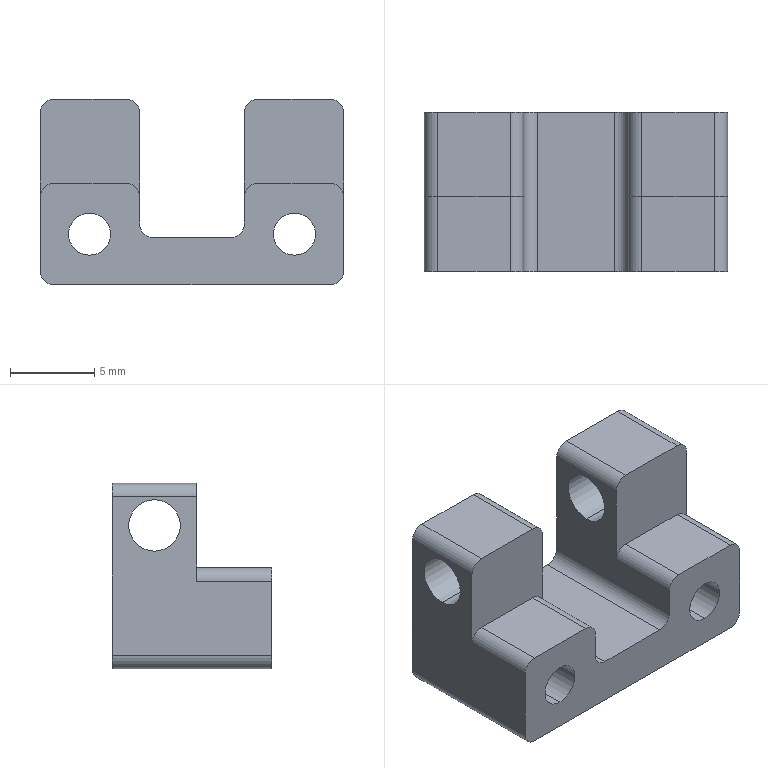Part | SolidWorks | features ICE 2, Extrusion 1, Fillet 1, HoleWzd 1 | 1 solid | 34 faces | box 18 x 9.45 x 11 mm | volume 943.932 mm3 | cylinder 20 | plane 14 | commonest cylinder face diameters 1.6 x12 2.5 x4 3.05 x4
STEP:
#1=CARTESIAN_POINT('',(-3.1,6.95,4.175));
#2=VERTEX_POINT('',#1);
#3=CARTESIAN_POINT('',(-3.1,6.95,7.225));
#4=VERTEX_POINT('',#3);
#5=CARTESIAN_POINT('',(-3.1,6.95,5.7));
#6=DIRECTION('',(-1.,0.,0.));
#7=DIRECTION('',(0.,0.,1.));
#8=AXIS2_PLACEMENT_3D('',#5,#6,#7);
#9=CIRCLE('',#8,1.525);
#10=EDGE_CURVE('',#2,#4,#9,.T.);
#11=ORIENTED_EDGE('',*,*,#10,.F.);
#12=CARTESIAN_POINT('',(-9.,6.95,4.175));
#13=VERTEX_POINT('',#12);
#14=CARTESIAN_POINT('',(9.,6.95,4.175));
#15=DIRECTION('',(-1.,0.,0.));
#16=VECTOR('',#15,1000.);
#17=LINE('',#14,#16);
#18=EDGE_CURVE('',#2,#13,#17,.T.);
#19=ORIENTED_EDGE('',*,*,#18,.T.);
#20=CARTESIAN_POINT('',(-9.,6.95,7.225));
#21=VERTEX_POINT('',#20);
#22=CARTESIAN_POINT('',(-9.,6.95,5.7));
#23=DIRECTION('',(-1.,0.,0.));
#24=DIRECTION('',(0.,0.,1.));
#25=AXIS2_PLACEMENT_3D('',#22,#23,#24);
#26=CIRCLE('',#25,1.525);
#27=EDGE_CURVE('',#13,#21,#26,.T.);
#28=ORIENTED_EDGE('',*,*,#27,.T.);
#29=CARTESIAN_POINT('',(9.,6.95,7.225));
#30=DIRECTION('',(-1.,0.,0.));
#31=VECTOR('',#30,1000.);
#32=LINE('',#29,#31);
#33=EDGE_CURVE('',#4,#21,#32,.T.);
#34=ORIENTED_EDGE('',*,*,#33,.F.);
#35=EDGE_LOOP('',(#11,#19,#28,#34));
#36=FACE_OUTER_BOUND('',#35,.T.);
#37=CARTESIAN_POINT('',(9.,6.95,5.7));
#38=DIRECTION('',(-1.,0.,0.));
#39=DIRECTION('',(0.,0.,1.));
#40=AXIS2_PLACEMENT_3D('',#37,#38,#39);
#41=CYLINDRICAL_SURFACE('',#40,1.525);
#42=ADVANCED_FACE('',(#36),#41,.F.);
#43=CARTESIAN_POINT('',(9.,6.95,4.175));
#44=VERTEX_POINT('',#43);
#45=CARTESIAN_POINT('',(9.,6.95,7.225));
#46=VERTEX_POINT('',#45);
#47=CARTESIAN_POINT('',(9.,6.95,5.7));
#48=DIRECTION('',(-1.,0.,0.));
#49=DIRECTION('',(0.,0.,1.));
#50=AXIS2_PLACEMENT_3D('',#47,#48,#49);
#51=CIRCLE('',#50,1.525);
#52=EDGE_CURVE('',#44,#46,#51,.T.);
#53=ORIENTED_EDGE('',*,*,#52,.F.);
#54=CARTESIAN_POINT('',(3.1,6.95,4.175));
#55=VERTEX_POINT('',#54);
#56=CARTESIAN_POINT('',(9.,6.95,4.175));
#57=DIRECTION('',(-1.,0.,0.));
#58=VECTOR('',#57,1000.);
#59=LINE('',#56,#58);
#60=EDGE_CURVE('',#44,#55,#59,.T.);
#61=ORIENTED_EDGE('',*,*,#60,.T.);
#62=CARTESIAN_POINT('',(3.1,6.95,7.225));
#63=VERTEX_POINT('',#62);
#64=CARTESIAN_POINT('',(3.1,6.95,5.7));
#65=DIRECTION('',(1.,0.,0.));
#66=DIRECTION('',(0.,0.,-1.));
#67=AXIS2_PLACEMENT_3D('',#64,#65,#66);
#68=CIRCLE('',#67,1.525);
#69=EDGE_CURVE('',#63,#55,#68,.T.);
#70=ORIENTED_EDGE('',*,*,#69,.F.);
#71=CARTESIAN_POINT('',(9.,6.95,7.225));
#72=DIRECTION('',(-1.,0.,0.));
#73=VECTOR('',#72,1000.);
#74=LINE('',#71,#73);
#75=EDGE_CURVE('',#46,#63,#74,.T.);
#76=ORIENTED_EDGE('',*,*,#75,.F.);
#77=EDGE_LOOP('',(#53,#61,#70,#76));
#78=FACE_OUTER_BOUND('',#77,.T.);
#79=CARTESIAN_POINT('',(9.,6.95,5.7));
#80=DIRECTION('',(-1.,0.,0.));
#81=DIRECTION('',(0.,0.,1.));
#82=AXIS2_PLACEMENT_3D('',#79,#80,#81);
#83=CYLINDRICAL_SURFACE('',#82,1.525);
#84=ADVANCED_FACE('',(#78),#83,.F.);
#85=CARTESIAN_POINT('',(-6.075,9.45,1.45));
#86=VERTEX_POINT('',#85);
#87=CARTESIAN_POINT('',(-6.075,9.45,-1.05));
#88=VERTEX_POINT('',#87);
#89=CARTESIAN_POINT('',(-6.075,9.45,0.2));
#90=DIRECTION('',(0.,-1.,0.));
#91=DIRECTION('',(0.,0.,-1.));
#92=AXIS2_PLACEMENT_3D('',#89,#90,#91);
#93=CIRCLE('',#92,1.25);
#94=EDGE_CURVE('',#86,#88,#93,.T.);
#95=ORIENTED_EDGE('',*,*,#94,.F.);
#96=CARTESIAN_POINT('',(-6.075,0.,1.45));
#97=VERTEX_POINT('',#96);
#98=CARTESIAN_POINT('',(-6.075,0.,1.45));
#99=DIRECTION('',(0.,-1.,0.));
#100=VECTOR('',#99,1000.);
#101=LINE('',#98,#100);
#102=EDGE_CURVE('',#86,#97,#101,.T.);
#103=ORIENTED_EDGE('',*,*,#102,.T.);
#104=CARTESIAN_POINT('',(-6.075,0.,-1.05));
#105=VERTEX_POINT('',#104);
#106=CARTESIAN_POINT('',(-6.075,0.,0.2));
#107=DIRECTION('',(0.,-1.,0.));
#108=DIRECTION('',(0.,0.,-1.));
#109=AXIS2_PLACEMENT_3D('',#106,#107,#108);
#110=CIRCLE('',#109,1.25);
#111=EDGE_CURVE('',#97,#105,#110,.T.);
#112=ORIENTED_EDGE('',*,*,#111,.T.);
#113=CARTESIAN_POINT('',(-6.075,0.,-1.05));
#114=DIRECTION('',(0.,-1.,0.));
#115=VECTOR('',#114,1000.);
#116=LINE('',#113,#115);
#117=EDGE_CURVE('',#88,#105,#116,.T.);
#118=ORIENTED_EDGE('',*,*,#117,.F.);
#119=EDGE_LOOP('',(#95,#103,#112,#118));
#120=FACE_OUTER_BOUND('',#119,.T.);
#121=CARTESIAN_POINT('',(-6.075,0.,0.2));
#122=DIRECTION('',(0.,-1.,0.));
#123=DIRECTION('',(0.,0.,-1.));
#124=AXIS2_PLACEMENT_3D('',#121,#122,#123);
#125=CYLINDRICAL_SURFACE('',#124,1.25);
#126=ADVANCED_FACE('',(#120),#125,.F.);
#127=CARTESIAN_POINT('',(6.075,9.45,1.45));
#128=VERTEX_POINT('',#127);
#129=CARTESIAN_POINT('',(6.075,9.45,-1.05));
#130=VERTEX_POINT('',#129);
#131=CARTESIAN_POINT('',(6.075,9.45,0.2));
#132=DIRECTION('',(0.,-1.,0.));
#133=DIRECTION('',(0.,0.,-1.));
#134=AXIS2_PLACEMENT_3D('',#131,#132,#133);
#135=CIRCLE('',#134,1.25);
#136=EDGE_CURVE('',#128,#130,#135,.T.);
#137=ORIENTED_EDGE('',*,*,#136,.F.);
#138=CARTESIAN_POINT('',(6.075,0.,1.45));
#139=VERTEX_POINT('',#138);
#140=CARTESIAN_POINT('',(6.075,0.,1.45));
#141=DIRECTION('',(0.,-1.,0.));
#142=VECTOR('',#141,1000.);
#143=LINE('',#140,#142);
#144=EDGE_CURVE('',#128,#139,#143,.T.);
#145=ORIENTED_EDGE('',*,*,#144,.T.);
#146=CARTESIAN_POINT('',(6.075,0.,-1.05));
#147=VERTEX_POINT('',#146);
#148=CARTESIAN_POINT('',(6.075,0.,0.2));
#149=DIRECTION('',(0.,-1.,0.));
#150=DIRECTION('',(0.,0.,-1.));
#151=AXIS2_PLACEMENT_3D('',#148,#149,#150);
#152=CIRCLE('',#151,1.25);
#153=EDGE_CURVE('',#139,#147,#152,.T.);
#154=ORIENTED_EDGE('',*,*,#153,.T.);
#155=CARTESIAN_POINT('',(6.075,0.,-1.05));
#156=DIRECTION('',(0.,-1.,0.));
#157=VECTOR('',#156,1000.);
#158=LINE('',#155,#157);
#159=EDGE_CURVE('',#130,#147,#158,.T.);
#160=ORIENTED_EDGE('',*,*,#159,.F.);
#161=EDGE_LOOP('',(#137,#145,#154,#160));
#162=FACE_OUTER_BOUND('',#161,.T.);
#163=CARTESIAN_POINT('',(6.075,0.,0.2));
#164=DIRECTION('',(0.,-1.,0.));
#165=DIRECTION('',(0.,0.,-1.));
#166=AXIS2_PLACEMENT_3D('',#163,#164,#165);
#167=CYLINDRICAL_SURFACE('',#166,1.25);
#168=ADVANCED_FACE('',(#162),#167,.F.);
#169=CARTESIAN_POINT('',(-9.,6.95,5.7));
#170=DIRECTION('',(-1.,0.,0.));
#171=DIRECTION('',(0.,0.,1.));
#172=AXIS2_PLACEMENT_3D('',#169,#170,#171);
#173=CIRCLE('',#172,1.525);
#174=EDGE_CURVE('',#21,#13,#173,.T.);
#175=ORIENTED_EDGE('',*,*,#174,.F.);
#176=ORIENTED_EDGE('',*,*,#27,.F.);
#177=EDGE_LOOP('',(#175,#176));
#178=FACE_BOUND('',#177,.T.);
#179=CARTESIAN_POINT('',(-9.,0.,-2.));
#180=VERTEX_POINT('',#179);
#181=CARTESIAN_POINT('',(-9.,0.,2.4));
#182=VERTEX_POINT('',#181);
#183=CARTESIAN_POINT('',(-9.,0.,3.2));
#184=DIRECTION('',(0.,0.,1.));
#185=VECTOR('',#184,1000.);
#186=LINE('',#183,#185);
#187=EDGE_CURVE('',#180,#182,#186,.T.);
#188=ORIENTED_EDGE('',*,*,#187,.T.);
#189=CARTESIAN_POINT('',(-9.,4.45,2.4));
#190=VERTEX_POINT('',#189);
#191=CARTESIAN_POINT('',(-9.,4.45,2.4));
#192=DIRECTION('',(0.,1.,0.));
#193=VECTOR('',#192,1000.);
#194=LINE('',#191,#193);
#195=EDGE_CURVE('',#182,#190,#194,.T.);
#196=ORIENTED_EDGE('',*,*,#195,.T.);
#197=CARTESIAN_POINT('',(-9.,4.45,7.4));
#198=VERTEX_POINT('',#197);
#199=CARTESIAN_POINT('',(-9.,4.45,-2.8));
#200=DIRECTION('',(0.,0.,1.));
#201=VECTOR('',#200,1000.);
#202=LINE('',#199,#201);
#203=EDGE_CURVE('',#190,#198,#202,.T.);
#204=ORIENTED_EDGE('',*,*,#203,.T.);
#205=CARTESIAN_POINT('',(-9.,9.45,7.4));
#206=VERTEX_POINT('',#205);
#207=CARTESIAN_POINT('',(-9.,4.45,7.4));
#208=DIRECTION('',(0.,1.,0.));
#209=VECTOR('',#208,1000.);
#210=LINE('',#207,#209);
#211=EDGE_CURVE('',#198,#206,#210,.T.);
#212=ORIENTED_EDGE('',*,*,#211,.T.);
#213=CARTESIAN_POINT('',(-9.,9.45,-2.));
#214=VERTEX_POINT('',#213);
#215=CARTESIAN_POINT('',(-9.,9.45,-2.8));
#216=DIRECTION('',(0.,0.,1.));
#217=VECTOR('',#216,1000.);
#218=LINE('',#215,#217);
#219=EDGE_CURVE('',#214,#206,#218,.T.);
#220=ORIENTED_EDGE('',*,*,#219,.F.);
#221=CARTESIAN_POINT('',(-9.,4.45,-2.));
#222=DIRECTION('',(0.,-1.,0.));
#223=VECTOR('',#222,1000.);
#224=LINE('',#221,#223);
#225=EDGE_CURVE('',#214,#180,#224,.T.);
#226=ORIENTED_EDGE('',*,*,#225,.T.);
#227=EDGE_LOOP('',(#188,#196,#204,#212,#220,#226));
#228=FACE_OUTER_BOUND('',#227,.T.);
#229=CARTESIAN_POINT('',(-9.,4.45,3.2));
#230=DIRECTION('',(1.,0.,0.));
#231=DIRECTION('',(0.,0.,-1.));
#232=AXIS2_PLACEMENT_3D('',#229,#230,#231);
#233=PLANE('',#232);
#234=ADVANCED_FACE('',(#178,#228),#233,.F.);
#235=CARTESIAN_POINT('',(-8.2,4.45,3.2));
#236=VERTEX_POINT('',#235);
#237=CARTESIAN_POINT('',(-3.9,4.45,3.2));
#238=VERTEX_POINT('',#237);
#239=CARTESIAN_POINT('',(-3.1,4.45,3.2));
#240=DIRECTION('',(1.,0.,0.));
#241=VECTOR('',#240,1000.);
#242=LINE('',#239,#241);
#243=EDGE_CURVE('',#236,#238,#242,.T.);
#244=ORIENTED_EDGE('',*,*,#243,.F.);
#245=CARTESIAN_POINT('',(-8.2,0.,3.2));
#246=VERTEX_POINT('',#245);
#247=CARTESIAN_POINT('',(-8.2,4.45,3.2));
#248=DIRECTION('',(0.,-1.,0.));
#249=VECTOR('',#248,1000.);
#250=LINE('',#247,#249);
#251=EDGE_CURVE('',#236,#246,#250,.T.);
#252=ORIENTED_EDGE('',*,*,#251,.T.);
#253=CARTESIAN_POINT('',(-3.9,0.,3.2));
#254=VERTEX_POINT('',#253);
#255=CARTESIAN_POINT('',(-3.1,0.,3.2));
#256=DIRECTION('',(1.,0.,0.));
#257=VECTOR('',#256,1000.);
#258=LINE('',#255,#257);
#259=EDGE_CURVE('',#246,#254,#258,.T.);
#260=ORIENTED_EDGE('',*,*,#259,.T.);
#261=CARTESIAN_POINT('',(-3.9,4.45,3.2));
#262=DIRECTION('',(0.,1.,0.));
#263=VECTOR('',#262,1000.);
#264=LINE('',#261,#263);
#265=EDGE_CURVE('',#254,#238,#264,.T.);
#266=ORIENTED_EDGE('',*,*,#265,.T.);
#267=EDGE_LOOP('',(#244,#252,#260,#266));
#268=FACE_OUTER_BOUND('',#267,.T.);
#269=CARTESIAN_POINT('',(-3.1,4.45,3.2));
#270=DIRECTION('',(0.,0.,-1.));
#271=DIRECTION('',(-1.,0.,0.));
#272=AXIS2_PLACEMENT_3D('',#269,#270,#271);
#273=PLANE('',#272);
#274=ADVANCED_FACE('',(#268),#273,.F.);
#275=CARTESIAN_POINT('',(-3.1,6.95,5.7));
#276=DIRECTION('',(-1.,0.,0.));
#277=DIRECTION('',(0.,0.,1.));
#278=AXIS2_PLACEMENT_3D('',#275,#276,#277);
#279=CIRCLE('',#278,1.525);
#280=EDGE_CURVE('',#4,#2,#279,.T.);
#281=ORIENTED_EDGE('',*,*,#280,.T.);
#282=ORIENTED_EDGE('',*,*,#10,.T.);
#283=EDGE_LOOP('',(#281,#282));
#284=FACE_BOUND('',#283,.T.);
#285=CARTESIAN_POINT('',(-3.1,4.45,7.4));
#286=VERTEX_POINT('',#285);
#287=CARTESIAN_POINT('',(-3.1,4.45,2.4));
#288=VERTEX_POINT('',#287);
#289=CARTESIAN_POINT('',(-3.1,4.45,8.2));
#290=DIRECTION('',(0.,0.,-1.));
#291=VECTOR('',#290,1000.);
#292=LINE('',#289,#291);
#293=EDGE_CURVE('',#286,#288,#292,.T.);
#294=ORIENTED_EDGE('',*,*,#293,.T.);
#295=CARTESIAN_POINT('',(-3.1,0.,2.4));
#296=VERTEX_POINT('',#295);
#297=CARTESIAN_POINT('',(-3.1,4.45,2.4));
#298=DIRECTION('',(0.,-1.,0.));
#299=VECTOR('',#298,1000.);
#300=LINE('',#297,#299);
#301=EDGE_CURVE('',#288,#296,#300,.T.);
#302=ORIENTED_EDGE('',*,*,#301,.T.);
#303=CARTESIAN_POINT('',(-3.1,0.,0.8));
#304=VERTEX_POINT('',#303);
#305=CARTESIAN_POINT('',(-3.1,0.,0.));
#306=DIRECTION('',(0.,0.,-1.));
#307=VECTOR('',#306,1000.);
#308=LINE('',#305,#307);
#309=EDGE_CURVE('',#296,#304,#308,.T.);
#310=ORIENTED_EDGE('',*,*,#309,.T.);
#311=CARTESIAN_POINT('',(-3.1,9.45,0.8));
#312=VERTEX_POINT('',#311);
#313=CARTESIAN_POINT('',(-3.1,9.45,0.8));
#314=DIRECTION('',(0.,1.,0.));
#315=VECTOR('',#314,1000.);
#316=LINE('',#313,#315);
#317=EDGE_CURVE('',#304,#312,#316,.T.);
#318=ORIENTED_EDGE('',*,*,#317,.T.);
#319=CARTESIAN_POINT('',(-3.1,9.45,7.4));
#320=VERTEX_POINT('',#319);
#321=CARTESIAN_POINT('',(-3.1,9.45,8.2));
#322=DIRECTION('',(0.,0.,-1.));
#323=VECTOR('',#322,1000.);
#324=LINE('',#321,#323);
#325=EDGE_CURVE('',#320,#312,#324,.T.);
#326=ORIENTED_EDGE('',*,*,#325,.F.);
#327=CARTESIAN_POINT('',(-3.1,4.45,7.4));
#328=DIRECTION('',(0.,-1.,0.));
#329=VECTOR('',#328,1000.);
#330=LINE('',#327,#329);
#331=EDGE_CURVE('',#320,#286,#330,.T.);
#332=ORIENTED_EDGE('',*,*,#331,.T.);
#333=EDGE_LOOP('',(#294,#302,#310,#318,#326,#332));
#334=FACE_OUTER_BOUND('',#333,.T.);
#335=CARTESIAN_POINT('',(-3.1,4.45,0.));
#336=DIRECTION('',(-1.,0.,0.));
#337=DIRECTION('',(0.,0.,1.));
#338=AXIS2_PLACEMENT_3D('',#335,#336,#337);
#339=PLANE('',#338);
#340=ADVANCED_FACE('',(#284,#334),#339,.F.);
#341=CARTESIAN_POINT('',(-2.3,0.,0.));
#342=VERTEX_POINT('',#341);
#343=CARTESIAN_POINT('',(2.3,0.,0.));
#344=VERTEX_POINT('',#343);
#345=CARTESIAN_POINT('',(3.1,0.,0.));
#346=DIRECTION('',(1.,0.,0.));
#347=VECTOR('',#346,1000.);
#348=LINE('',#345,#347);
#349=EDGE_CURVE('',#342,#344,#348,.T.);
#350=ORIENTED_EDGE('',*,*,#349,.T.);
#351=CARTESIAN_POINT('',(2.3,9.45,0.));
#352=VERTEX_POINT('',#351);
#353=CARTESIAN_POINT('',(2.3,9.45,0.));
#354=DIRECTION('',(0.,1.,0.));
#355=VECTOR('',#354,1000.);
#356=LINE('',#353,#355);
#357=EDGE_CURVE('',#344,#352,#356,.T.);
#358=ORIENTED_EDGE('',*,*,#357,.T.);
#359=CARTESIAN_POINT('',(-2.3,9.45,0.));
#360=VERTEX_POINT('',#359);
#361=CARTESIAN_POINT('',(-3.1,9.45,0.));
#362=DIRECTION('',(1.,0.,0.));
#363=VECTOR('',#362,1000.);
#364=LINE('',#361,#363);
#365=EDGE_CURVE('',#360,#352,#364,.T.);
#366=ORIENTED_EDGE('',*,*,#365,.F.);
#367=CARTESIAN_POINT('',(-2.3,0.,0.));
#368=DIRECTION('',(0.,-1.,0.));
#369=VECTOR('',#368,1000.);
#370=LINE('',#367,#369);
#371=EDGE_CURVE('',#360,#342,#370,.T.);
#372=ORIENTED_EDGE('',*,*,#371,.T.);
#373=EDGE_LOOP('',(#350,#358,#366,#372));
#374=FACE_OUTER_BOUND('',#373,.T.);
#375=CARTESIAN_POINT('',(3.1,4.45,0.));
#376=DIRECTION('',(0.,0.,-1.));
#377=DIRECTION('',(-1.,0.,0.));
#378=AXIS2_PLACEMENT_3D('',#375,#376,#377);
#379=PLANE('',#378);
#380=ADVANCED_FACE('',(#374),#379,.F.);
#381=ORIENTED_EDGE('',*,*,#69,.T.);
#382=CARTESIAN_POINT('',(3.1,6.95,5.7));
#383=DIRECTION('',(1.,0.,0.));
#384=DIRECTION('',(0.,0.,-1.));
#385=AXIS2_PLACEMENT_3D('',#382,#383,#384);
#386=CIRCLE('',#385,1.525);
#387=EDGE_CURVE('',#55,#63,#386,.T.);
#388=ORIENTED_EDGE('',*,*,#387,.T.);
#389=EDGE_LOOP('',(#381,#388));
#390=FACE_BOUND('',#389,.T.);
#391=CARTESIAN_POINT('',(3.1,0.,0.8));
#392=VERTEX_POINT('',#391);
#393=CARTESIAN_POINT('',(3.1,0.,2.4));
#394=VERTEX_POINT('',#393);
#395=CARTESIAN_POINT('',(3.1,0.,3.2));
#396=DIRECTION('',(0.,0.,1.));
#397=VECTOR('',#396,1000.);
#398=LINE('',#395,#397);
#399=EDGE_CURVE('',#392,#394,#398,.T.);
#400=ORIENTED_EDGE('',*,*,#399,.T.);
#401=CARTESIAN_POINT('',(3.1,4.45,2.4));
#402=VERTEX_POINT('',#401);
#403=CARTESIAN_POINT('',(3.1,4.45,2.4));
#404=DIRECTION('',(0.,1.,0.));
#405=VECTOR('',#404,1000.);
#406=LINE('',#403,#405);
#407=EDGE_CURVE('',#394,#402,#406,.T.);
#408=ORIENTED_EDGE('',*,*,#407,.T.);
#409=CARTESIAN_POINT('',(3.1,4.45,7.4));
#410=VERTEX_POINT('',#409);
#411=CARTESIAN_POINT('',(3.1,4.45,0.));
#412=DIRECTION('',(0.,0.,1.));
#413=VECTOR('',#412,1000.);
#414=LINE('',#411,#413);
#415=EDGE_CURVE('',#402,#410,#414,.T.);
#416=ORIENTED_EDGE('',*,*,#415,.T.);
#417=CARTESIAN_POINT('',(3.1,9.45,7.4));
#418=VERTEX_POINT('',#417);
#419=CARTESIAN_POINT('',(3.1,4.45,7.4));
#420=DIRECTION('',(0.,1.,0.));
#421=VECTOR('',#420,1000.);
#422=LINE('',#419,#421);
#423=EDGE_CURVE('',#410,#418,#422,.T.);
#424=ORIENTED_EDGE('',*,*,#423,.T.);
#425=CARTESIAN_POINT('',(3.1,9.45,0.8));
#426=VERTEX_POINT('',#425);
#427=CARTESIAN_POINT('',(3.1,9.45,0.));
#428=DIRECTION('',(0.,0.,1.));
#429=VECTOR('',#428,1000.);
#430=LINE('',#427,#429);
#431=EDGE_CURVE('',#426,#418,#430,.T.);
#432=ORIENTED_EDGE('',*,*,#431,.F.);
#433=CARTESIAN_POINT('',(3.1,0.,0.8));
#434=DIRECTION('',(0.,-1.,0.));
#435=VECTOR('',#434,1000.);
#436=LINE('',#433,#435);
#437=EDGE_CURVE('',#426,#392,#436,.T.);
#438=ORIENTED_EDGE('',*,*,#437,.T.);
#439=EDGE_LOOP('',(#400,#408,#416,#424,#432,#438));
#440=FACE_OUTER_BOUND('',#439,.T.);
#441=CARTESIAN_POINT('',(3.1,4.45,3.2));
#442=DIRECTION('',(1.,0.,0.));
#443=DIRECTION('',(0.,0.,-1.));
#444=AXIS2_PLACEMENT_3D('',#441,#442,#443);
#445=PLANE('',#444);
#446=ADVANCED_FACE('',(#390,#440),#445,.F.);
#447=CARTESIAN_POINT('',(3.9,4.45,3.2));
#448=VERTEX_POINT('',#447);
#449=CARTESIAN_POINT('',(8.2,4.45,3.2));
#450=VERTEX_POINT('',#449);
#451=CARTESIAN_POINT('',(9.,4.45,3.2));
#452=DIRECTION('',(1.,0.,0.));
#453=VECTOR('',#452,1000.);
#454=LINE('',#451,#453);
#455=EDGE_CURVE('',#448,#450,#454,.T.);
#456=ORIENTED_EDGE('',*,*,#455,.F.);
#457=CARTESIAN_POINT('',(3.9,0.,3.2));
#458=VERTEX_POINT('',#457);
#459=CARTESIAN_POINT('',(3.9,4.45,3.2));
#460=DIRECTION('',(0.,-1.,0.));
#461=VECTOR('',#460,1000.);
#462=LINE('',#459,#461);
#463=EDGE_CURVE('',#448,#458,#462,.T.);
#464=ORIENTED_EDGE('',*,*,#463,.T.);
#465=CARTESIAN_POINT('',(8.2,0.,3.2));
#466=VERTEX_POINT('',#465);
#467=CARTESIAN_POINT('',(9.,0.,3.2));
#468=DIRECTION('',(1.,0.,0.));
#469=VECTOR('',#468,1000.);
#470=LINE('',#467,#469);
#471=EDGE_CURVE('',#458,#466,#470,.T.);
#472=ORIENTED_EDGE('',*,*,#471,.T.);
#473=CARTESIAN_POINT('',(8.2,4.45,3.2));
#474=DIRECTION('',(0.,1.,0.));
#475=VECTOR('',#474,1000.);
#476=LINE('',#473,#475);
#477=EDGE_CURVE('',#466,#450,#476,.T.);
#478=ORIENTED_EDGE('',*,*,#477,.T.);
#479=EDGE_LOOP('',(#456,#464,#472,#478));
#480=FACE_OUTER_BOUND('',#479,.T.);
#481=CARTESIAN_POINT('',(9.,4.45,3.2));
#482=DIRECTION('',(0.,0.,-1.));
#483=DIRECTION('',(-1.,0.,0.));
#484=AXIS2_PLACEMENT_3D('',#481,#482,#483);
#485=PLANE('',#484);
#486=ADVANCED_FACE('',(#480),#485,.F.);
#487=CARTESIAN_POINT('',(9.,6.95,5.7));
#488=DIRECTION('',(-1.,0.,0.));
#489=DIRECTION('',(0.,0.,1.));
#490=AXIS2_PLACEMENT_3D('',#487,#488,#489);
#491=CIRCLE('',#490,1.525);
#492=EDGE_CURVE('',#46,#44,#491,.T.);
#493=ORIENTED_EDGE('',*,*,#492,.T.);
#494=ORIENTED_EDGE('',*,*,#52,.T.);
#495=EDGE_LOOP('',(#493,#494));
#496=FACE_BOUND('',#495,.T.);
#497=CARTESIAN_POINT('',(9.,4.45,7.4));
#498=VERTEX_POINT('',#497);
#499=CARTESIAN_POINT('',(9.,4.45,2.4));
#500=VERTEX_POINT('',#499);
#501=CARTESIAN_POINT('',(9.,4.45,8.2));
#502=DIRECTION('',(0.,0.,-1.));
#503=VECTOR('',#502,1000.);
#504=LINE('',#501,#503);
#505=EDGE_CURVE('',#498,#500,#504,.T.);
#506=ORIENTED_EDGE('',*,*,#505,.T.);
#507=CARTESIAN_POINT('',(9.,0.,2.4));
#508=VERTEX_POINT('',#507);
#509=CARTESIAN_POINT('',(9.,4.45,2.4));
#510=DIRECTION('',(0.,-1.,0.));
#511=VECTOR('',#510,1000.);
#512=LINE('',#509,#511);
#513=EDGE_CURVE('',#500,#508,#512,.T.);
#514=ORIENTED_EDGE('',*,*,#513,.T.);
#515=CARTESIAN_POINT('',(9.,0.,-2.));
#516=VERTEX_POINT('',#515);
#517=CARTESIAN_POINT('',(9.,0.,-2.8));
#518=DIRECTION('',(0.,0.,-1.));
#519=VECTOR('',#518,1000.);
#520=LINE('',#517,#519);
#521=EDGE_CURVE('',#508,#516,#520,.T.);
#522=ORIENTED_EDGE('',*,*,#521,.T.);
#523=CARTESIAN_POINT('',(9.,9.45,-2.));
#524=VERTEX_POINT('',#523);
#525=CARTESIAN_POINT('',(9.,4.45,-2.));
#526=DIRECTION('',(0.,1.,0.));
#527=VECTOR('',#526,1000.);
#528=LINE('',#525,#527);
#529=EDGE_CURVE('',#516,#524,#528,.T.);
#530=ORIENTED_EDGE('',*,*,#529,.T.);
#531=CARTESIAN_POINT('',(9.,9.45,7.4));
#532=VERTEX_POINT('',#531);
#533=CARTESIAN_POINT('',(9.,9.45,8.2));
#534=DIRECTION('',(0.,0.,-1.));
#535=VECTOR('',#534,1000.);
#536=LINE('',#533,#535);
#537=EDGE_CURVE('',#532,#524,#536,.T.);
#538=ORIENTED_EDGE('',*,*,#537,.F.);
#539=CARTESIAN_POINT('',(9.,4.45,7.4));
#540=DIRECTION('',(0.,-1.,0.));
#541=VECTOR('',#540,1000.);
#542=LINE('',#539,#541);
#543=EDGE_CURVE('',#532,#498,#542,.T.);
#544=ORIENTED_EDGE('',*,*,#543,.T.);
#545=EDGE_LOOP('',(#506,#514,#522,#530,#538,#544));
#546=FACE_OUTER_BOUND('',#545,.T.);
#547=CARTESIAN_POINT('',(9.,4.45,-2.8));
#548=DIRECTION('',(-1.,0.,0.));
#549=DIRECTION('',(0.,0.,1.));
#550=AXIS2_PLACEMENT_3D('',#547,#548,#549);
#551=PLANE('',#550);
#552=ADVANCED_FACE('',(#496,#546),#551,.F.);
#553=CARTESIAN_POINT('',(8.2,0.,-2.8));
#554=VERTEX_POINT('',#553);
#555=CARTESIAN_POINT('',(-8.2,0.,-2.8));
#556=VERTEX_POINT('',#555);
#557=CARTESIAN_POINT('',(-9.,0.,-2.8));
#558=DIRECTION('',(-1.,0.,0.));
#559=VECTOR('',#558,1000.);
#560=LINE('',#557,#559);
#561=EDGE_CURVE('',#554,#556,#560,.T.);
#562=ORIENTED_EDGE('',*,*,#561,.T.);
#563=CARTESIAN_POINT('',(-8.2,9.45,-2.8));
#564=VERTEX_POINT('',#563);
#565=CARTESIAN_POINT('',(-8.2,4.45,-2.8));
#566=DIRECTION('',(0.,1.,0.));
#567=VECTOR('',#566,1000.);
#568=LINE('',#565,#567);
#569=EDGE_CURVE('',#556,#564,#568,.T.);
#570=ORIENTED_EDGE('',*,*,#569,.T.);
#571=CARTESIAN_POINT('',(8.2,9.45,-2.8));
#572=VERTEX_POINT('',#571);
#573=CARTESIAN_POINT('',(9.,9.45,-2.8));
#574=DIRECTION('',(-1.,0.,0.));
#575=VECTOR('',#574,1000.);
#576=LINE('',#573,#575);
#577=EDGE_CURVE('',#572,#564,#576,.T.);
#578=ORIENTED_EDGE('',*,*,#577,.F.);
#579=CARTESIAN_POINT('',(8.2,4.45,-2.8));
#580=DIRECTION('',(0.,-1.,0.));
#581=VECTOR('',#580,1000.);
#582=LINE('',#579,#581);
#583=EDGE_CURVE('',#572,#554,#582,.T.);
#584=ORIENTED_EDGE('',*,*,#583,.T.);
#585=EDGE_LOOP('',(#562,#570,#578,#584));
#586=FACE_OUTER_BOUND('',#585,.T.);
#587=CARTESIAN_POINT('',(-9.,4.45,-2.8));
#588=DIRECTION('',(0.,0.,1.));
#589=DIRECTION('',(1.,0.,0.));
#590=AXIS2_PLACEMENT_3D('',#587,#588,#589);
#591=PLANE('',#590);
#592=ADVANCED_FACE('',(#586),#591,.F.);
#593=CARTESIAN_POINT('',(-6.075,0.,0.2));
#594=DIRECTION('',(0.,-1.,0.));
#595=DIRECTION('',(0.,0.,-1.));
#596=AXIS2_PLACEMENT_3D('',#593,#594,#595);
#597=CIRCLE('',#596,1.25);
#598=EDGE_CURVE('',#105,#97,#597,.T.);
#599=ORIENTED_EDGE('',*,*,#598,.F.);
#600=ORIENTED_EDGE('',*,*,#111,.F.);
#601=EDGE_LOOP('',(#599,#600));
#602=FACE_BOUND('',#601,.T.);
#603=CARTESIAN_POINT('',(6.075,0.,0.2));
#604=DIRECTION('',(0.,-1.,0.));
#605=DIRECTION('',(0.,0.,-1.));
#606=AXIS2_PLACEMENT_3D('',#603,#604,#605);
#607=CIRCLE('',#606,1.25);
#608=EDGE_CURVE('',#147,#139,#607,.T.);
#609=ORIENTED_EDGE('',*,*,#608,.F.);
#610=ORIENTED_EDGE('',*,*,#153,.F.);
#611=EDGE_LOOP('',(#609,#610));
#612=FACE_BOUND('',#611,.T.);
#613=ORIENTED_EDGE('',*,*,#259,.F.);
#614=CARTESIAN_POINT('',(-8.2,0.,2.4));
#615=DIRECTION('',(0.,-1.,0.));
#616=DIRECTION('',(0.,0.,-1.));
#617=AXIS2_PLACEMENT_3D('',#614,#615,#616);
#618=CIRCLE('',#617,0.8);
#619=EDGE_CURVE('',#246,#182,#618,.T.);
#620=ORIENTED_EDGE('',*,*,#619,.T.);
#621=ORIENTED_EDGE('',*,*,#187,.F.);
#622=CARTESIAN_POINT('',(-8.2,0.,-2.));
#623=DIRECTION('',(0.,-1.,0.));
#624=DIRECTION('',(0.,0.,-1.));
#625=AXIS2_PLACEMENT_3D('',#622,#623,#624);
#626=CIRCLE('',#625,0.8);
#627=EDGE_CURVE('',#180,#556,#626,.T.);
#628=ORIENTED_EDGE('',*,*,#627,.T.);
#629=ORIENTED_EDGE('',*,*,#561,.F.);
#630=CARTESIAN_POINT('',(8.2,0.,-2.));
#631=DIRECTION('',(0.,-1.,0.));
#632=DIRECTION('',(0.,0.,-1.));
#633=AXIS2_PLACEMENT_3D('',#630,#631,#632);
#634=CIRCLE('',#633,0.8);
#635=EDGE_CURVE('',#554,#516,#634,.T.);
#636=ORIENTED_EDGE('',*,*,#635,.T.);
#637=ORIENTED_EDGE('',*,*,#521,.F.);
#638=CARTESIAN_POINT('',(8.2,0.,2.4));
#639=DIRECTION('',(0.,-1.,0.));
#640=DIRECTION('',(0.,0.,-1.));
#641=AXIS2_PLACEMENT_3D('',#638,#639,#640);
#642=CIRCLE('',#641,0.8);
#643=EDGE_CURVE('',#508,#466,#642,.T.);
#644=ORIENTED_EDGE('',*,*,#643,.T.);
#645=ORIENTED_EDGE('',*,*,#471,.F.);
#646=CARTESIAN_POINT('',(3.9,0.,2.4));
#647=DIRECTION('',(0.,-1.,0.));
#648=DIRECTION('',(0.,0.,-1.));
#649=AXIS2_PLACEMENT_3D('',#646,#647,#648);
#650=CIRCLE('',#649,0.8);
#651=EDGE_CURVE('',#458,#394,#650,.T.);
#652=ORIENTED_EDGE('',*,*,#651,.T.);
#653=ORIENTED_EDGE('',*,*,#399,.F.);
#654=CARTESIAN_POINT('',(2.3,0.,0.8));
#655=DIRECTION('',(0.,1.,0.));
#656=DIRECTION('',(0.,0.,-1.));
#657=AXIS2_PLACEMENT_3D('',#654,#655,#656);
#658=CIRCLE('',#657,0.8);
#659=EDGE_CURVE('',#392,#344,#658,.T.);
#660=ORIENTED_EDGE('',*,*,#659,.T.);
#661=ORIENTED_EDGE('',*,*,#349,.F.);
#662=CARTESIAN_POINT('',(-2.3,0.,0.8));
#663=DIRECTION('',(0.,1.,0.));
#664=DIRECTION('',(0.,0.,-1.));
#665=AXIS2_PLACEMENT_3D('',#662,#663,#664);
#666=CIRCLE('',#665,0.8);
#667=EDGE_CURVE('',#342,#304,#666,.T.);
#668=ORIENTED_EDGE('',*,*,#667,.T.);
#669=ORIENTED_EDGE('',*,*,#309,.F.);
#670=CARTESIAN_POINT('',(-3.9,0.,2.4));
#671=DIRECTION('',(0.,-1.,0.));
#672=DIRECTION('',(0.,0.,-1.));
#673=AXIS2_PLACEMENT_3D('',#670,#671,#672);
#674=CIRCLE('',#673,0.8);
#675=EDGE_CURVE('',#296,#254,#674,.T.);
#676=ORIENTED_EDGE('',*,*,#675,.T.);
#677=EDGE_LOOP('',(#613,#620,#621,#628,#629,#636,#637,#644,#645,#652,#653,#660,#661,#668,#669,#676));
#678=FACE_OUTER_BOUND('',#677,.T.);
#679=CARTESIAN_POINT('',(0.,0.,0.));
#680=DIRECTION('',(0.,-1.,0.));
#681=DIRECTION('',(0.,0.,-1.));
#682=AXIS2_PLACEMENT_3D('',#679,#680,#681);
#683=PLANE('',#682);
#684=ADVANCED_FACE('',(#602,#612,#678),#683,.T.);
#685=ORIENTED_EDGE('',*,*,#293,.F.);
#686=CARTESIAN_POINT('',(-3.9,4.45,8.2));
#687=VERTEX_POINT('',#686);
#688=CARTESIAN_POINT('',(-3.9,4.45,7.4));
#689=DIRECTION('',(0.,-1.,0.));
#690=DIRECTION('',(0.,0.,1.));
#691=AXIS2_PLACEMENT_3D('',#688,#689,#690);
#692=CIRCLE('',#691,0.8);
#693=EDGE_CURVE('',#286,#687,#692,.T.);
#694=ORIENTED_EDGE('',*,*,#693,.T.);
#695=CARTESIAN_POINT('',(-8.2,4.45,8.2));
#696=VERTEX_POINT('',#695);
#697=CARTESIAN_POINT('',(-9.,4.45,8.2));
#698=DIRECTION('',(1.,0.,0.));
#699=VECTOR('',#698,1000.);
#700=LINE('',#697,#699);
#701=EDGE_CURVE('',#696,#687,#700,.T.);
#702=ORIENTED_EDGE('',*,*,#701,.F.);
#703=CARTESIAN_POINT('',(-8.2,4.45,7.4));
#704=DIRECTION('',(0.,-1.,0.));
#705=DIRECTION('',(0.,0.,1.));
#706=AXIS2_PLACEMENT_3D('',#703,#704,#705);
#707=CIRCLE('',#706,0.8);
#708=EDGE_CURVE('',#696,#198,#707,.T.);
#709=ORIENTED_EDGE('',*,*,#708,.T.);
#710=ORIENTED_EDGE('',*,*,#203,.F.);
#711=CARTESIAN_POINT('',(-8.2,4.45,2.4));
#712=DIRECTION('',(0.,1.,0.));
#713=DIRECTION('',(0.,0.,1.));
#714=AXIS2_PLACEMENT_3D('',#711,#712,#713);
#715=CIRCLE('',#714,0.8);
#716=EDGE_CURVE('',#190,#236,#715,.T.);
#717=ORIENTED_EDGE('',*,*,#716,.T.);
#718=ORIENTED_EDGE('',*,*,#243,.T.);
#719=CARTESIAN_POINT('',(-3.9,4.45,2.4));
#720=DIRECTION('',(0.,1.,0.));
#721=DIRECTION('',(0.,0.,1.));
#722=AXIS2_PLACEMENT_3D('',#719,#720,#721);
#723=CIRCLE('',#722,0.8);
#724=EDGE_CURVE('',#238,#288,#723,.T.);
#725=ORIENTED_EDGE('',*,*,#724,.T.);
#726=EDGE_LOOP('',(#685,#694,#702,#709,#710,#717,#718,#725));
#727=FACE_OUTER_BOUND('',#726,.T.);
#728=CARTESIAN_POINT('',(0.,4.45,0.));
#729=DIRECTION('',(0.,1.,0.));
#730=DIRECTION('',(0.,0.,1.));
#731=AXIS2_PLACEMENT_3D('',#728,#729,#730);
#732=PLANE('',#731);
#733=ADVANCED_FACE('',(#727),#732,.F.);
#734=ORIENTED_EDGE('',*,*,#505,.F.);
#735=CARTESIAN_POINT('',(8.2,4.45,8.2));
#736=VERTEX_POINT('',#735);
#737=CARTESIAN_POINT('',(8.2,4.45,7.4));
#738=DIRECTION('',(0.,-1.,0.));
#739=DIRECTION('',(0.,0.,1.));
#740=AXIS2_PLACEMENT_3D('',#737,#738,#739);
#741=CIRCLE('',#740,0.8);
#742=EDGE_CURVE('',#498,#736,#741,.T.);
#743=ORIENTED_EDGE('',*,*,#742,.T.);
#744=CARTESIAN_POINT('',(3.9,4.45,8.2));
#745=VERTEX_POINT('',#744);
#746=CARTESIAN_POINT('',(3.1,4.45,8.2));
#747=DIRECTION('',(1.,0.,0.));
#748=VECTOR('',#747,1000.);
#749=LINE('',#746,#748);
#750=EDGE_CURVE('',#745,#736,#749,.T.);
#751=ORIENTED_EDGE('',*,*,#750,.F.);
#752=CARTESIAN_POINT('',(3.9,4.45,7.4));
#753=DIRECTION('',(0.,-1.,0.));
#754=DIRECTION('',(0.,0.,1.));
#755=AXIS2_PLACEMENT_3D('',#752,#753,#754);
#756=CIRCLE('',#755,0.8);
#757=EDGE_CURVE('',#745,#410,#756,.T.);
#758=ORIENTED_EDGE('',*,*,#757,.T.);
#759=ORIENTED_EDGE('',*,*,#415,.F.);
#760=CARTESIAN_POINT('',(3.9,4.45,2.4));
#761=DIRECTION('',(0.,1.,0.));
#762=DIRECTION('',(0.,0.,1.));
#763=AXIS2_PLACEMENT_3D('',#760,#761,#762);
#764=CIRCLE('',#763,0.8);
#765=EDGE_CURVE('',#402,#448,#764,.T.);
#766=ORIENTED_EDGE('',*,*,#765,.T.);
#767=ORIENTED_EDGE('',*,*,#455,.T.);
#768=CARTESIAN_POINT('',(8.2,4.45,2.4));
#769=DIRECTION('',(0.,1.,0.));
#770=DIRECTION('',(0.,0.,1.));
#771=AXIS2_PLACEMENT_3D('',#768,#769,#770);
#772=CIRCLE('',#771,0.8);
#773=EDGE_CURVE('',#450,#500,#772,.T.);
#774=ORIENTED_EDGE('',*,*,#773,.T.);
#775=EDGE_LOOP('',(#734,#743,#751,#758,#759,#766,#767,#774));
#776=FACE_OUTER_BOUND('',#775,.T.);
#777=CARTESIAN_POINT('',(0.,4.45,0.));
#778=DIRECTION('',(0.,1.,0.));
#779=DIRECTION('',(0.,0.,1.));
#780=AXIS2_PLACEMENT_3D('',#777,#778,#779);
#781=PLANE('',#780);
#782=ADVANCED_FACE('',(#776),#781,.F.);
#783=ORIENTED_EDGE('',*,*,#701,.T.);
#784=CARTESIAN_POINT('',(-3.9,9.45,8.2));
#785=VERTEX_POINT('',#784);
#786=CARTESIAN_POINT('',(-3.9,9.45,8.2));
#787=DIRECTION('',(0.,1.,0.));
#788=VECTOR('',#787,1000.);
#789=LINE('',#786,#788);
#790=EDGE_CURVE('',#687,#785,#789,.T.);
#791=ORIENTED_EDGE('',*,*,#790,.T.);
#792=CARTESIAN_POINT('',(-8.2,9.45,8.2));
#793=VERTEX_POINT('',#792);
#794=CARTESIAN_POINT('',(-9.,9.45,8.2));
#795=DIRECTION('',(1.,0.,0.));
#796=VECTOR('',#795,1000.);
#797=LINE('',#794,#796);
#798=EDGE_CURVE('',#793,#785,#797,.T.);
#799=ORIENTED_EDGE('',*,*,#798,.F.);
#800=CARTESIAN_POINT('',(-8.2,9.45,8.2));
#801=DIRECTION('',(0.,-1.,0.));
#802=VECTOR('',#801,1000.);
#803=LINE('',#800,#802);
#804=EDGE_CURVE('',#793,#696,#803,.T.);
#805=ORIENTED_EDGE('',*,*,#804,.T.);
#806=EDGE_LOOP('',(#783,#791,#799,#805));
#807=FACE_OUTER_BOUND('',#806,.T.);
#808=CARTESIAN_POINT('',(-9.,9.45,8.2));
#809=DIRECTION('',(0.,0.,-1.));
#810=DIRECTION('',(-1.,0.,0.));
#811=AXIS2_PLACEMENT_3D('',#808,#809,#810);
#812=PLANE('',#811);
#813=ADVANCED_FACE('',(#807),#812,.F.);
#814=ORIENTED_EDGE('',*,*,#750,.T.);
#815=CARTESIAN_POINT('',(8.2,9.45,8.2));
#816=VERTEX_POINT('',#815);
#817=CARTESIAN_POINT('',(8.2,9.45,8.2));
#818=DIRECTION('',(0.,1.,0.));
#819=VECTOR('',#818,1000.);
#820=LINE('',#817,#819);
#821=EDGE_CURVE('',#736,#816,#820,.T.);
#822=ORIENTED_EDGE('',*,*,#821,.T.);
#823=CARTESIAN_POINT('',(3.9,9.45,8.2));
#824=VERTEX_POINT('',#823);
#825=CARTESIAN_POINT('',(3.1,9.45,8.2));
#826=DIRECTION('',(1.,0.,0.));
#827=VECTOR('',#826,1000.);
#828=LINE('',#825,#827);
#829=EDGE_CURVE('',#824,#816,#828,.T.);
#830=ORIENTED_EDGE('',*,*,#829,.F.);
#831=CARTESIAN_POINT('',(3.9,9.45,8.2));
#832=DIRECTION('',(0.,-1.,0.));
#833=VECTOR('',#832,1000.);
#834=LINE('',#831,#833);
#835=EDGE_CURVE('',#824,#745,#834,.T.);
#836=ORIENTED_EDGE('',*,*,#835,.T.);
#837=EDGE_LOOP('',(#814,#822,#830,#836));
#838=FACE_OUTER_BOUND('',#837,.T.);
#839=CARTESIAN_POINT('',(3.1,9.45,8.2));
#840=DIRECTION('',(0.,0.,-1.));
#841=DIRECTION('',(-1.,0.,0.));
#842=AXIS2_PLACEMENT_3D('',#839,#840,#841);
#843=PLANE('',#842);
#844=ADVANCED_FACE('',(#838),#843,.F.);
#845=CARTESIAN_POINT('',(-6.075,9.45,0.2));
#846=DIRECTION('',(0.,-1.,0.));
#847=DIRECTION('',(0.,0.,-1.));
#848=AXIS2_PLACEMENT_3D('',#845,#846,#847);
#849=CIRCLE('',#848,1.25);
#850=EDGE_CURVE('',#88,#86,#849,.T.);
#851=ORIENTED_EDGE('',*,*,#850,.T.);
#852=ORIENTED_EDGE('',*,*,#94,.T.);
#853=EDGE_LOOP('',(#851,#852));
#854=FACE_BOUND('',#853,.T.);
#855=CARTESIAN_POINT('',(6.075,9.45,0.2));
#856=DIRECTION('',(0.,-1.,0.));
#857=DIRECTION('',(0.,0.,-1.));
#858=AXIS2_PLACEMENT_3D('',#855,#856,#857);
#859=CIRCLE('',#858,1.25);
#860=EDGE_CURVE('',#130,#128,#859,.T.);
#861=ORIENTED_EDGE('',*,*,#860,.T.);
#862=ORIENTED_EDGE('',*,*,#136,.T.);
#863=EDGE_LOOP('',(#861,#862));
#864=FACE_BOUND('',#863,.T.);
#865=ORIENTED_EDGE('',*,*,#577,.T.);
#866=CARTESIAN_POINT('',(-8.2,9.45,-2.));
#867=DIRECTION('',(0.,1.,0.));
#868=DIRECTION('',(0.,0.,1.));
#869=AXIS2_PLACEMENT_3D('',#866,#867,#868);
#870=CIRCLE('',#869,0.8);
#871=EDGE_CURVE('',#564,#214,#870,.T.);
#872=ORIENTED_EDGE('',*,*,#871,.T.);
#873=ORIENTED_EDGE('',*,*,#219,.T.);
#874=CARTESIAN_POINT('',(-8.2,9.45,7.4));
#875=DIRECTION('',(0.,1.,0.));
#876=DIRECTION('',(0.,0.,1.));
#877=AXIS2_PLACEMENT_3D('',#874,#875,#876);
#878=CIRCLE('',#877,0.8);
#879=EDGE_CURVE('',#206,#793,#878,.T.);
#880=ORIENTED_EDGE('',*,*,#879,.T.);
#881=ORIENTED_EDGE('',*,*,#798,.T.);
#882=CARTESIAN_POINT('',(-3.9,9.45,7.4));
#883=DIRECTION('',(0.,1.,0.));
#884=DIRECTION('',(0.,0.,1.));
#885=AXIS2_PLACEMENT_3D('',#882,#883,#884);
#886=CIRCLE('',#885,0.8);
#887=EDGE_CURVE('',#785,#320,#886,.T.);
#888=ORIENTED_EDGE('',*,*,#887,.T.);
#889=ORIENTED_EDGE('',*,*,#325,.T.);
#890=CARTESIAN_POINT('',(-2.3,9.45,0.8));
#891=DIRECTION('',(0.,-1.,0.));
#892=DIRECTION('',(0.,0.,1.));
#893=AXIS2_PLACEMENT_3D('',#890,#891,#892);
#894=CIRCLE('',#893,0.8);
#895=EDGE_CURVE('',#312,#360,#894,.T.);
#896=ORIENTED_EDGE('',*,*,#895,.T.);
#897=ORIENTED_EDGE('',*,*,#365,.T.);
#898=CARTESIAN_POINT('',(2.3,9.45,0.8));
#899=DIRECTION('',(0.,-1.,0.));
#900=DIRECTION('',(0.,0.,1.));
#901=AXIS2_PLACEMENT_3D('',#898,#899,#900);
#902=CIRCLE('',#901,0.8);
#903=EDGE_CURVE('',#352,#426,#902,.T.);
#904=ORIENTED_EDGE('',*,*,#903,.T.);
#905=ORIENTED_EDGE('',*,*,#431,.T.);
#906=CARTESIAN_POINT('',(3.9,9.45,7.4));
#907=DIRECTION('',(0.,1.,0.));
#908=DIRECTION('',(0.,0.,1.));
#909=AXIS2_PLACEMENT_3D('',#906,#907,#908);
#910=CIRCLE('',#909,0.8);
#911=EDGE_CURVE('',#418,#824,#910,.T.);
#912=ORIENTED_EDGE('',*,*,#911,.T.);
#913=ORIENTED_EDGE('',*,*,#829,.T.);
#914=CARTESIAN_POINT('',(8.2,9.45,7.4));
#915=DIRECTION('',(0.,1.,0.));
#916=DIRECTION('',(0.,0.,1.));
#917=AXIS2_PLACEMENT_3D('',#914,#915,#916);
#918=CIRCLE('',#917,0.8);
#919=EDGE_CURVE('',#816,#532,#918,.T.);
#920=ORIENTED_EDGE('',*,*,#919,.T.);
#921=ORIENTED_EDGE('',*,*,#537,.T.);
#922=CARTESIAN_POINT('',(8.2,9.45,-2.));
#923=DIRECTION('',(0.,1.,0.));
#924=DIRECTION('',(0.,0.,1.));
#925=AXIS2_PLACEMENT_3D('',#922,#923,#924);
#926=CIRCLE('',#925,0.8);
#927=EDGE_CURVE('',#524,#572,#926,.T.);
#928=ORIENTED_EDGE('',*,*,#927,.T.);
#929=EDGE_LOOP('',(#865,#872,#873,#880,#881,#888,#889,#896,#897,#904,#905,#912,#913,#920,#921,#928));
#930=FACE_OUTER_BOUND('',#929,.T.);
#931=CARTESIAN_POINT('',(0.,9.45,0.));
#932=DIRECTION('',(0.,1.,0.));
#933=DIRECTION('',(0.,0.,1.));
#934=AXIS2_PLACEMENT_3D('',#931,#932,#933);
#935=PLANE('',#934);
#936=ADVANCED_FACE('',(#854,#864,#930),#935,.T.);
#937=ORIENTED_EDGE('',*,*,#144,.F.);
#938=ORIENTED_EDGE('',*,*,#860,.F.);
#939=ORIENTED_EDGE('',*,*,#159,.T.);
#940=ORIENTED_EDGE('',*,*,#608,.T.);
#941=EDGE_LOOP('',(#937,#938,#939,#940));
#942=FACE_OUTER_BOUND('',#941,.T.);
#943=CARTESIAN_POINT('',(6.075,0.,0.2));
#944=DIRECTION('',(0.,-1.,0.));
#945=DIRECTION('',(0.,0.,-1.));
#946=AXIS2_PLACEMENT_3D('',#943,#944,#945);
#947=CYLINDRICAL_SURFACE('',#946,1.25);
#948=ADVANCED_FACE('',(#942),#947,.F.);
#949=ORIENTED_EDGE('',*,*,#102,.F.);
#950=ORIENTED_EDGE('',*,*,#850,.F.);
#951=ORIENTED_EDGE('',*,*,#117,.T.);
#952=ORIENTED_EDGE('',*,*,#598,.T.);
#953=EDGE_LOOP('',(#949,#950,#951,#952));
#954=FACE_OUTER_BOUND('',#953,.T.);
#955=CARTESIAN_POINT('',(-6.075,0.,0.2));
#956=DIRECTION('',(0.,-1.,0.));
#957=DIRECTION('',(0.,0.,-1.));
#958=AXIS2_PLACEMENT_3D('',#955,#956,#957);
#959=CYLINDRICAL_SURFACE('',#958,1.25);
#960=ADVANCED_FACE('',(#954),#959,.F.);
#961=ORIENTED_EDGE('',*,*,#60,.F.);
#962=ORIENTED_EDGE('',*,*,#492,.F.);
#963=ORIENTED_EDGE('',*,*,#75,.T.);
#964=ORIENTED_EDGE('',*,*,#387,.F.);
#965=EDGE_LOOP('',(#961,#962,#963,#964));
#966=FACE_OUTER_BOUND('',#965,.T.);
#967=CARTESIAN_POINT('',(9.,6.95,5.7));
#968=DIRECTION('',(-1.,0.,0.));
#969=DIRECTION('',(0.,0.,1.));
#970=AXIS2_PLACEMENT_3D('',#967,#968,#969);
#971=CYLINDRICAL_SURFACE('',#970,1.525);
#972=ADVANCED_FACE('',(#966),#971,.F.);
#973=ORIENTED_EDGE('',*,*,#18,.F.);
#974=ORIENTED_EDGE('',*,*,#280,.F.);
#975=ORIENTED_EDGE('',*,*,#33,.T.);
#976=ORIENTED_EDGE('',*,*,#174,.T.);
#977=EDGE_LOOP('',(#973,#974,#975,#976));
#978=FACE_OUTER_BOUND('',#977,.T.);
#979=CARTESIAN_POINT('',(9.,6.95,5.7));
#980=DIRECTION('',(-1.,0.,0.));
#981=DIRECTION('',(0.,0.,1.));
#982=AXIS2_PLACEMENT_3D('',#979,#980,#981);
#983=CYLINDRICAL_SURFACE('',#982,1.525);
#984=ADVANCED_FACE('',(#978),#983,.F.);
#985=ORIENTED_EDGE('',*,*,#716,.F.);
#986=ORIENTED_EDGE('',*,*,#195,.F.);
#987=ORIENTED_EDGE('',*,*,#619,.F.);
#988=ORIENTED_EDGE('',*,*,#251,.F.);
#989=EDGE_LOOP('',(#985,#986,#987,#988));
#990=FACE_OUTER_BOUND('',#989,.T.);
#991=CARTESIAN_POINT('',(-8.2,4.45,2.4));
#992=DIRECTION('',(0.,-1.,0.));
#993=DIRECTION('',(0.,0.,-1.));
#994=AXIS2_PLACEMENT_3D('',#991,#992,#993);
#995=CYLINDRICAL_SURFACE('',#994,0.8);
#996=ADVANCED_FACE('',(#990),#995,.T.);
#997=ORIENTED_EDGE('',*,*,#724,.F.);
#998=ORIENTED_EDGE('',*,*,#265,.F.);
#999=ORIENTED_EDGE('',*,*,#675,.F.);
#1000=ORIENTED_EDGE('',*,*,#301,.F.);
#1001=EDGE_LOOP('',(#997,#998,#999,#1000));
#1002=FACE_OUTER_BOUND('',#1001,.T.);
#1003=CARTESIAN_POINT('',(-3.9,4.45,2.4));
#1004=DIRECTION('',(0.,-1.,0.));
#1005=DIRECTION('',(0.,0.,-1.));
#1006=AXIS2_PLACEMENT_3D('',#1003,#1004,#1005);
#1007=CYLINDRICAL_SURFACE('',#1006,0.8);
#1008=ADVANCED_FACE('',(#1002),#1007,.T.);
#1009=ORIENTED_EDGE('',*,*,#765,.F.);
#1010=ORIENTED_EDGE('',*,*,#407,.F.);
#1011=ORIENTED_EDGE('',*,*,#651,.F.);
#1012=ORIENTED_EDGE('',*,*,#463,.F.);
#1013=EDGE_LOOP('',(#1009,#1010,#1011,#1012));
#1014=FACE_OUTER_BOUND('',#1013,.T.);
#1015=CARTESIAN_POINT('',(3.9,4.45,2.4));
#1016=DIRECTION('',(0.,-1.,0.));
#1017=DIRECTION('',(0.,0.,-1.));
#1018=AXIS2_PLACEMENT_3D('',#1015,#1016,#1017);
#1019=CYLINDRICAL_SURFACE('',#1018,0.8);
#1020=ADVANCED_FACE('',(#1014),#1019,.T.);
#1021=ORIENTED_EDGE('',*,*,#773,.F.);
#1022=ORIENTED_EDGE('',*,*,#477,.F.);
#1023=ORIENTED_EDGE('',*,*,#643,.F.);
#1024=ORIENTED_EDGE('',*,*,#513,.F.);
#1025=EDGE_LOOP('',(#1021,#1022,#1023,#1024));
#1026=FACE_OUTER_BOUND('',#1025,.T.);
#1027=CARTESIAN_POINT('',(8.2,4.45,2.4));
#1028=DIRECTION('',(0.,-1.,0.));
#1029=DIRECTION('',(0.,0.,-1.));
#1030=AXIS2_PLACEMENT_3D('',#1027,#1028,#1029);
#1031=CYLINDRICAL_SURFACE('',#1030,0.8);
#1032=ADVANCED_FACE('',(#1026),#1031,.T.);
#1033=ORIENTED_EDGE('',*,*,#903,.F.);
#1034=ORIENTED_EDGE('',*,*,#357,.F.);
#1035=ORIENTED_EDGE('',*,*,#659,.F.);
#1036=ORIENTED_EDGE('',*,*,#437,.F.);
#1037=EDGE_LOOP('',(#1033,#1034,#1035,#1036));
#1038=FACE_OUTER_BOUND('',#1037,.T.);
#1039=CARTESIAN_POINT('',(2.3,4.45,0.8));
#1040=DIRECTION('',(0.,1.,0.));
#1041=DIRECTION('',(0.,0.,1.));
#1042=AXIS2_PLACEMENT_3D('',#1039,#1040,#1041);
#1043=CYLINDRICAL_SURFACE('',#1042,0.8);
#1044=ADVANCED_FACE('',(#1038),#1043,.F.);
#1045=ORIENTED_EDGE('',*,*,#895,.F.);
#1046=ORIENTED_EDGE('',*,*,#317,.F.);
#1047=ORIENTED_EDGE('',*,*,#667,.F.);
#1048=ORIENTED_EDGE('',*,*,#371,.F.);
#1049=EDGE_LOOP('',(#1045,#1046,#1047,#1048));
#1050=FACE_OUTER_BOUND('',#1049,.T.);
#1051=CARTESIAN_POINT('',(-2.3,4.45,0.8));
#1052=DIRECTION('',(0.,1.,0.));
#1053=DIRECTION('',(0.,0.,1.));
#1054=AXIS2_PLACEMENT_3D('',#1051,#1052,#1053);
#1055=CYLINDRICAL_SURFACE('',#1054,0.8);
#1056=ADVANCED_FACE('',(#1050),#1055,.F.);
#1057=ORIENTED_EDGE('',*,*,#871,.F.);
#1058=ORIENTED_EDGE('',*,*,#569,.F.);
#1059=ORIENTED_EDGE('',*,*,#627,.F.);
#1060=ORIENTED_EDGE('',*,*,#225,.F.);
#1061=EDGE_LOOP('',(#1057,#1058,#1059,#1060));
#1062=FACE_OUTER_BOUND('',#1061,.T.);
#1063=CARTESIAN_POINT('',(-8.2,4.45,-2.));
#1064=DIRECTION('',(0.,-1.,0.));
#1065=DIRECTION('',(0.,0.,-1.));
#1066=AXIS2_PLACEMENT_3D('',#1063,#1064,#1065);
#1067=CYLINDRICAL_SURFACE('',#1066,0.8);
#1068=ADVANCED_FACE('',(#1062),#1067,.T.);
#1069=ORIENTED_EDGE('',*,*,#927,.F.);
#1070=ORIENTED_EDGE('',*,*,#529,.F.);
#1071=ORIENTED_EDGE('',*,*,#635,.F.);
#1072=ORIENTED_EDGE('',*,*,#583,.F.);
#1073=EDGE_LOOP('',(#1069,#1070,#1071,#1072));
#1074=FACE_OUTER_BOUND('',#1073,.T.);
#1075=CARTESIAN_POINT('',(8.2,4.45,-2.));
#1076=DIRECTION('',(0.,-1.,0.));
#1077=DIRECTION('',(0.,0.,-1.));
#1078=AXIS2_PLACEMENT_3D('',#1075,#1076,#1077);
#1079=CYLINDRICAL_SURFACE('',#1078,0.8);
#1080=ADVANCED_FACE('',(#1074),#1079,.T.);
#1081=ORIENTED_EDGE('',*,*,#919,.F.);
#1082=ORIENTED_EDGE('',*,*,#821,.F.);
#1083=ORIENTED_EDGE('',*,*,#742,.F.);
#1084=ORIENTED_EDGE('',*,*,#543,.F.);
#1085=EDGE_LOOP('',(#1081,#1082,#1083,#1084));
#1086=FACE_OUTER_BOUND('',#1085,.T.);
#1087=CARTESIAN_POINT('',(8.2,4.45,7.4));
#1088=DIRECTION('',(0.,-1.,0.));
#1089=DIRECTION('',(0.,0.,-1.));
#1090=AXIS2_PLACEMENT_3D('',#1087,#1088,#1089);
#1091=CYLINDRICAL_SURFACE('',#1090,0.8);
#1092=ADVANCED_FACE('',(#1086),#1091,.T.);
#1093=ORIENTED_EDGE('',*,*,#911,.F.);
#1094=ORIENTED_EDGE('',*,*,#423,.F.);
#1095=ORIENTED_EDGE('',*,*,#757,.F.);
#1096=ORIENTED_EDGE('',*,*,#835,.F.);
#1097=EDGE_LOOP('',(#1093,#1094,#1095,#1096));
#1098=FACE_OUTER_BOUND('',#1097,.T.);
#1099=CARTESIAN_POINT('',(3.9,9.45,7.4));
#1100=DIRECTION('',(0.,-1.,0.));
#1101=DIRECTION('',(0.,0.,-1.));
#1102=AXIS2_PLACEMENT_3D('',#1099,#1100,#1101);
#1103=CYLINDRICAL_SURFACE('',#1102,0.8);
#1104=ADVANCED_FACE('',(#1098),#1103,.T.);
#1105=ORIENTED_EDGE('',*,*,#887,.F.);
#1106=ORIENTED_EDGE('',*,*,#790,.F.);
#1107=ORIENTED_EDGE('',*,*,#693,.F.);
#1108=ORIENTED_EDGE('',*,*,#331,.F.);
#1109=EDGE_LOOP('',(#1105,#1106,#1107,#1108));
#1110=FACE_OUTER_BOUND('',#1109,.T.);
#1111=CARTESIAN_POINT('',(-3.9,4.45,7.4));
#1112=DIRECTION('',(0.,-1.,0.));
#1113=DIRECTION('',(0.,0.,-1.));
#1114=AXIS2_PLACEMENT_3D('',#1111,#1112,#1113);
#1115=CYLINDRICAL_SURFACE('',#1114,0.8);
#1116=ADVANCED_FACE('',(#1110),#1115,.T.);
#1117=ORIENTED_EDGE('',*,*,#879,.F.);
#1118=ORIENTED_EDGE('',*,*,#211,.F.);
#1119=ORIENTED_EDGE('',*,*,#708,.F.);
#1120=ORIENTED_EDGE('',*,*,#804,.F.);
#1121=EDGE_LOOP('',(#1117,#1118,#1119,#1120));
#1122=FACE_OUTER_BOUND('',#1121,.T.);
#1123=CARTESIAN_POINT('',(-8.2,9.45,7.4));
#1124=DIRECTION('',(0.,-1.,0.));
#1125=DIRECTION('',(0.,0.,-1.));
#1126=AXIS2_PLACEMENT_3D('',#1123,#1124,#1125);
#1127=CYLINDRICAL_SURFACE('',#1126,0.8);
#1128=ADVANCED_FACE('',(#1122),#1127,.T.);
#1129=CLOSED_SHELL('',(#42,#84,#126,#168,#234,#274,#340,#380,#446,#486,#552,#592,#684,#733,#782,#813,#844,#936,#948,#960,#972,#984,#996,#1008,#1020,#1032,#1044,#1056,#1068,#1080,#1092,#1104,#1116,#1128));
#1130=MANIFOLD_SOLID_BREP('',#1129);
#1131=CARTESIAN_POINT('',(0.,0.,0.));
#1132=DIRECTION('',(0.,0.,1.));
#1133=DIRECTION('',(1.,0.,0.));
#1134=AXIS2_PLACEMENT_3D('',#1131,#1132,#1133);
#1135=(LENGTH_UNIT()NAMED_UNIT(*)SI_UNIT(.MILLI.,.METRE.));
#1136=UNCERTAINTY_MEASURE_WITH_UNIT(LENGTH_MEASURE(0.00001),#1135,'','');
#1137=(NAMED_UNIT(*)PLANE_ANGLE_UNIT()SI_UNIT($,.RADIAN.));
#1138=(NAMED_UNIT(*)SI_UNIT($,.STERADIAN.)SOLID_ANGLE_UNIT());
#1139=(GEOMETRIC_REPRESENTATION_CONTEXT(3)GLOBAL_UNCERTAINTY_ASSIGNED_CONTEXT((#1136))GLOBAL_UNIT_ASSIGNED_CONTEXT((#1135,#1137,#1138))REPRESENTATION_CONTEXT('',''));
#1140=ADVANCED_BREP_SHAPE_REPRESENTATION('',(#1130,#1134),#1139);